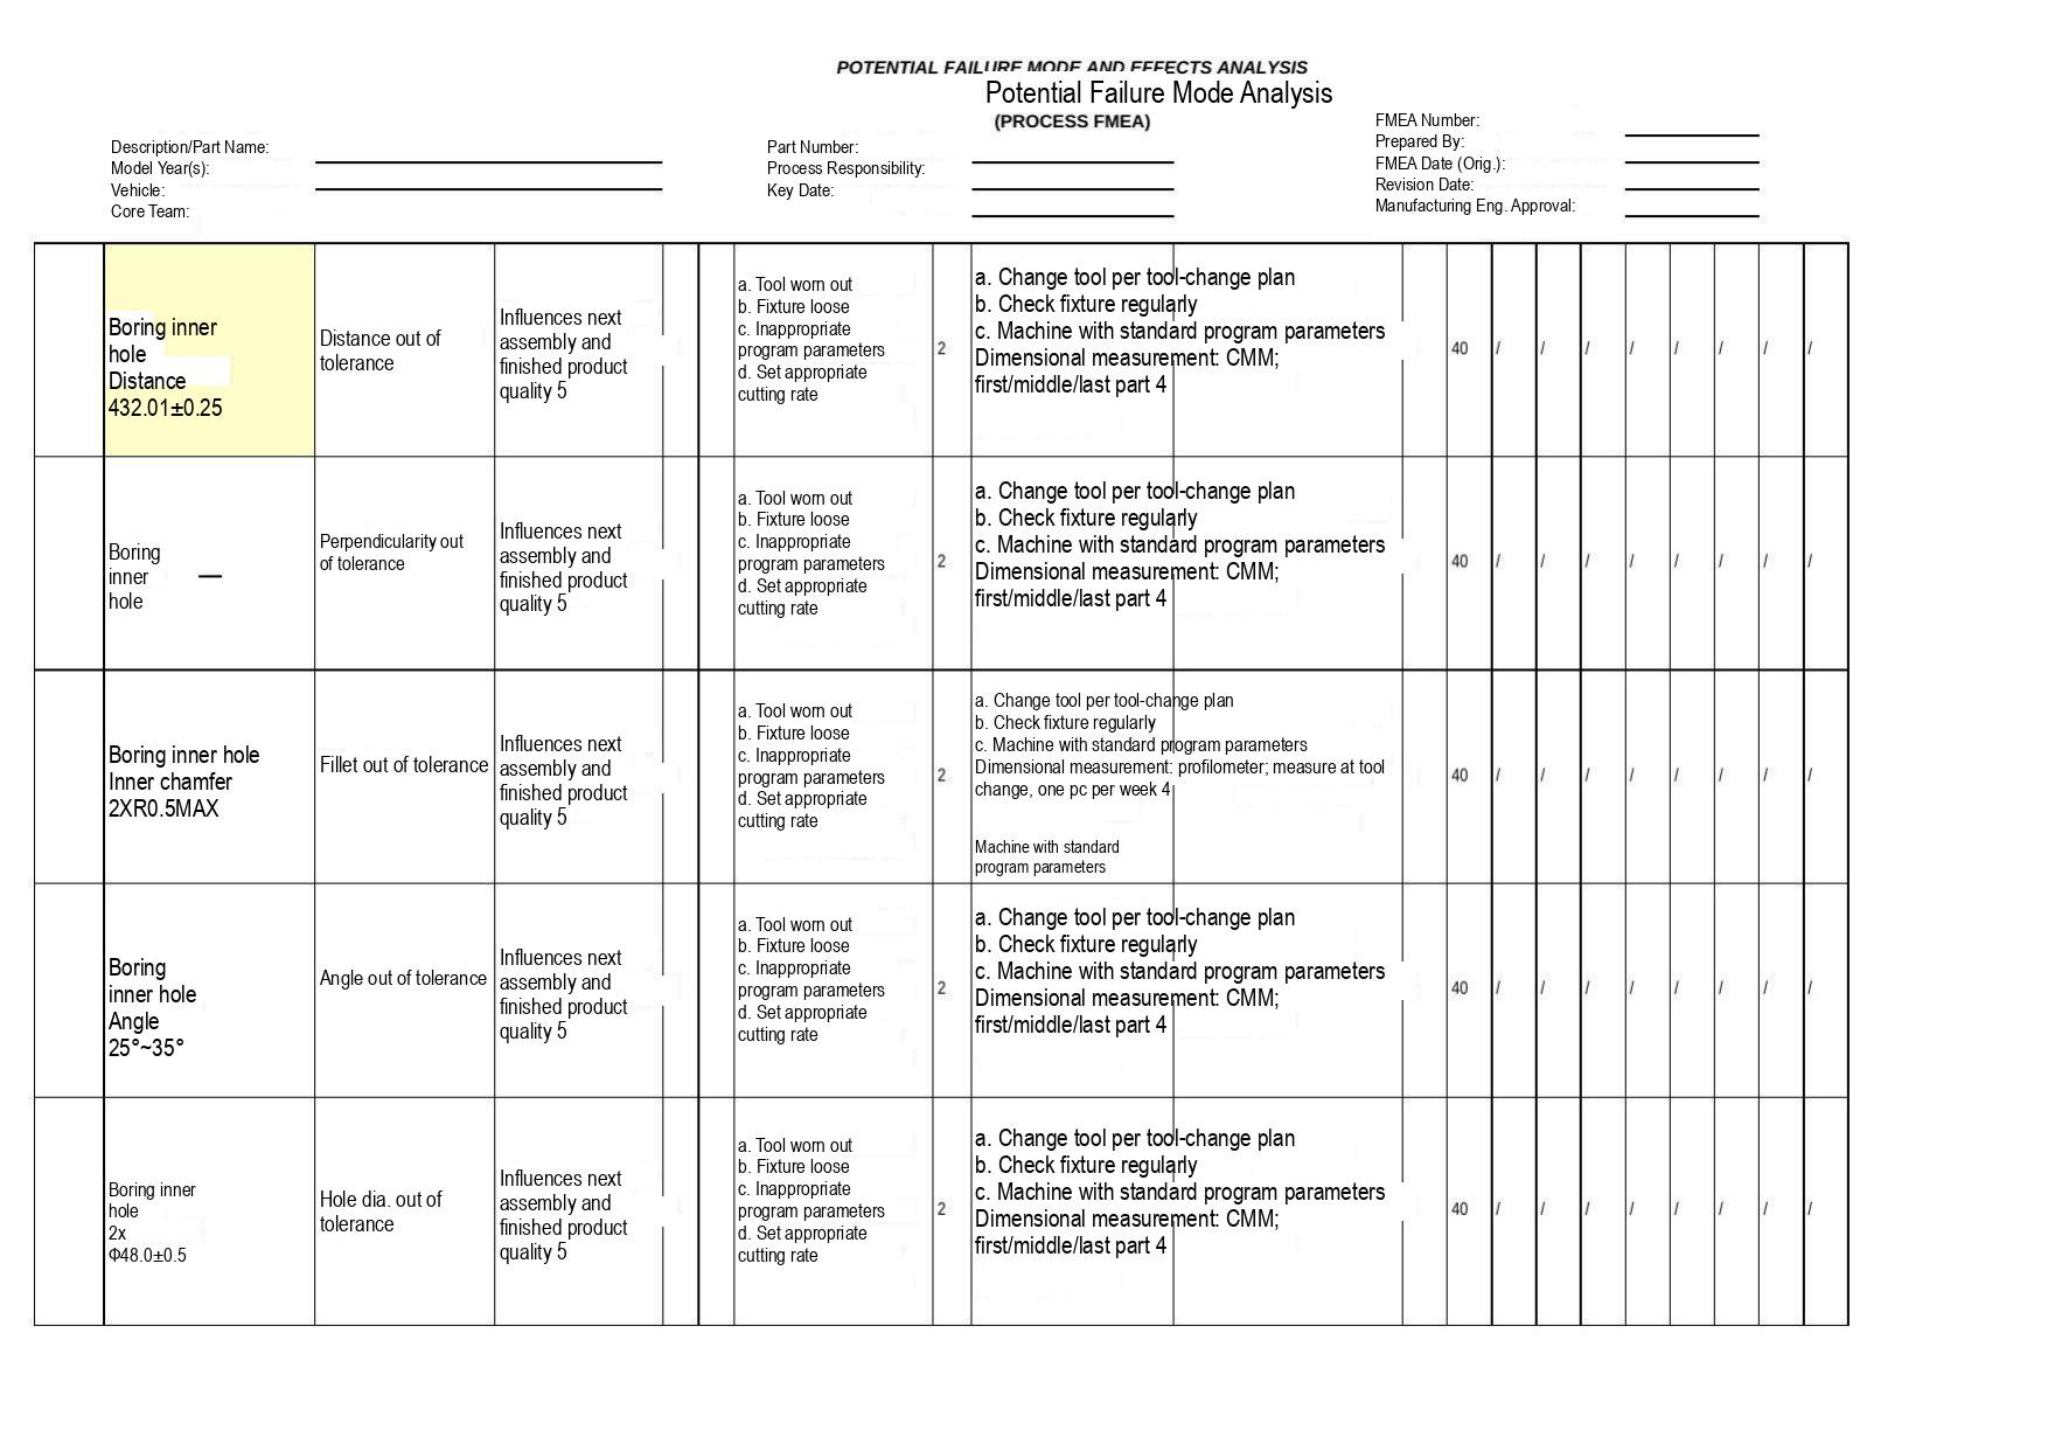**POTENTIAL FAILURE MODE AND EFFECTS ANALYSIS**

Potential Failure Mode Analysis

**(PROCESS FMEA)**

Description/Part Name:
Model Year(s):
Vehicle:
Core Team:

Part Number:
Process Responsibility:
Key Date:

FMEA Number:
Prepared By:
FMEA Date (Orig.):
Revision Date:
Manufacturing Eng. Approval:

| | | | | | | | | | | | | | | | | | | | |
|---|---|---|---|---|---|---|---|---|---|---|---|---|---|---|---|---|---|---|---|
| | Boring inner hole Distance 432.01±0.25 | Distance out of tolerance | Influences next assembly and finished product quality 5 | | | a. Tool worn out<br>b. Fixture loose<br>c. Inappropriate program parameters<br>d. Set appropriate cutting rate | 2 | a. Change tool per tool-change plan<br>b. Check fixture regularly<br>c. Machine with standard program parameters<br>Dimensional measurement: CMM; first/middle/last part 4 | | | 40 | / | / | / | / | / | / | / | / |
| | Boring inner hole — | Perpendicularity out of tolerance | Influences next assembly and finished product quality 5 | | | a. Tool worn out<br>b. Fixture loose<br>c. Inappropriate program parameters<br>d. Set appropriate cutting rate | 2 | a. Change tool per tool-change plan<br>b. Check fixture regularly<br>c. Machine with standard program parameters<br>Dimensional measurement: CMM; first/middle/last part 4 | | | 40 | / | / | / | / | / | / | / | / |
| | Boring inner hole Inner chamfer 2XR0.5MAX | Fillet out of tolerance | Influences next assembly and finished product quality 5 | | | a. Tool worn out<br>b. Fixture loose<br>c. Inappropriate program parameters<br>d. Set appropriate cutting rate | 2 | a. Change tool per tool-change plan<br>b. Check fixture regularly<br>c. Machine with standard program parameters<br>Dimensional measurement: profilometer; measure at tool change, one pc per week 4<br><br>Machine with standard program parameters | | | 40 | / | / | / | / | / | / | / | / |
| | Boring inner hole Angle 25°~35° | Angle out of tolerance | Influences next assembly and finished product quality 5 | | | a. Tool worn out<br>b. Fixture loose<br>c. Inappropriate program parameters<br>d. Set appropriate cutting rate | 2 | a. Change tool per tool-change plan<br>b. Check fixture regularly<br>c. Machine with standard program parameters<br>Dimensional measurement: CMM; first/middle/last part 4 | | | 40 | / | / | / | / | / | / | / | / |
| | Boring inner hole 2x Φ48.0±0.5 | Hole dia. out of tolerance | Influences next assembly and finished product quality 5 | | | a. Tool worn out<br>b. Fixture loose<br>c. Inappropriate program parameters<br>d. Set appropriate cutting rate | 2 | a. Change tool per tool-change plan<br>b. Check fixture regularly<br>c. Machine with standard program parameters<br>Dimensional measurement: CMM; first/middle/last part 4 | | | 40 | / | / | / | / | / | / | / | / |
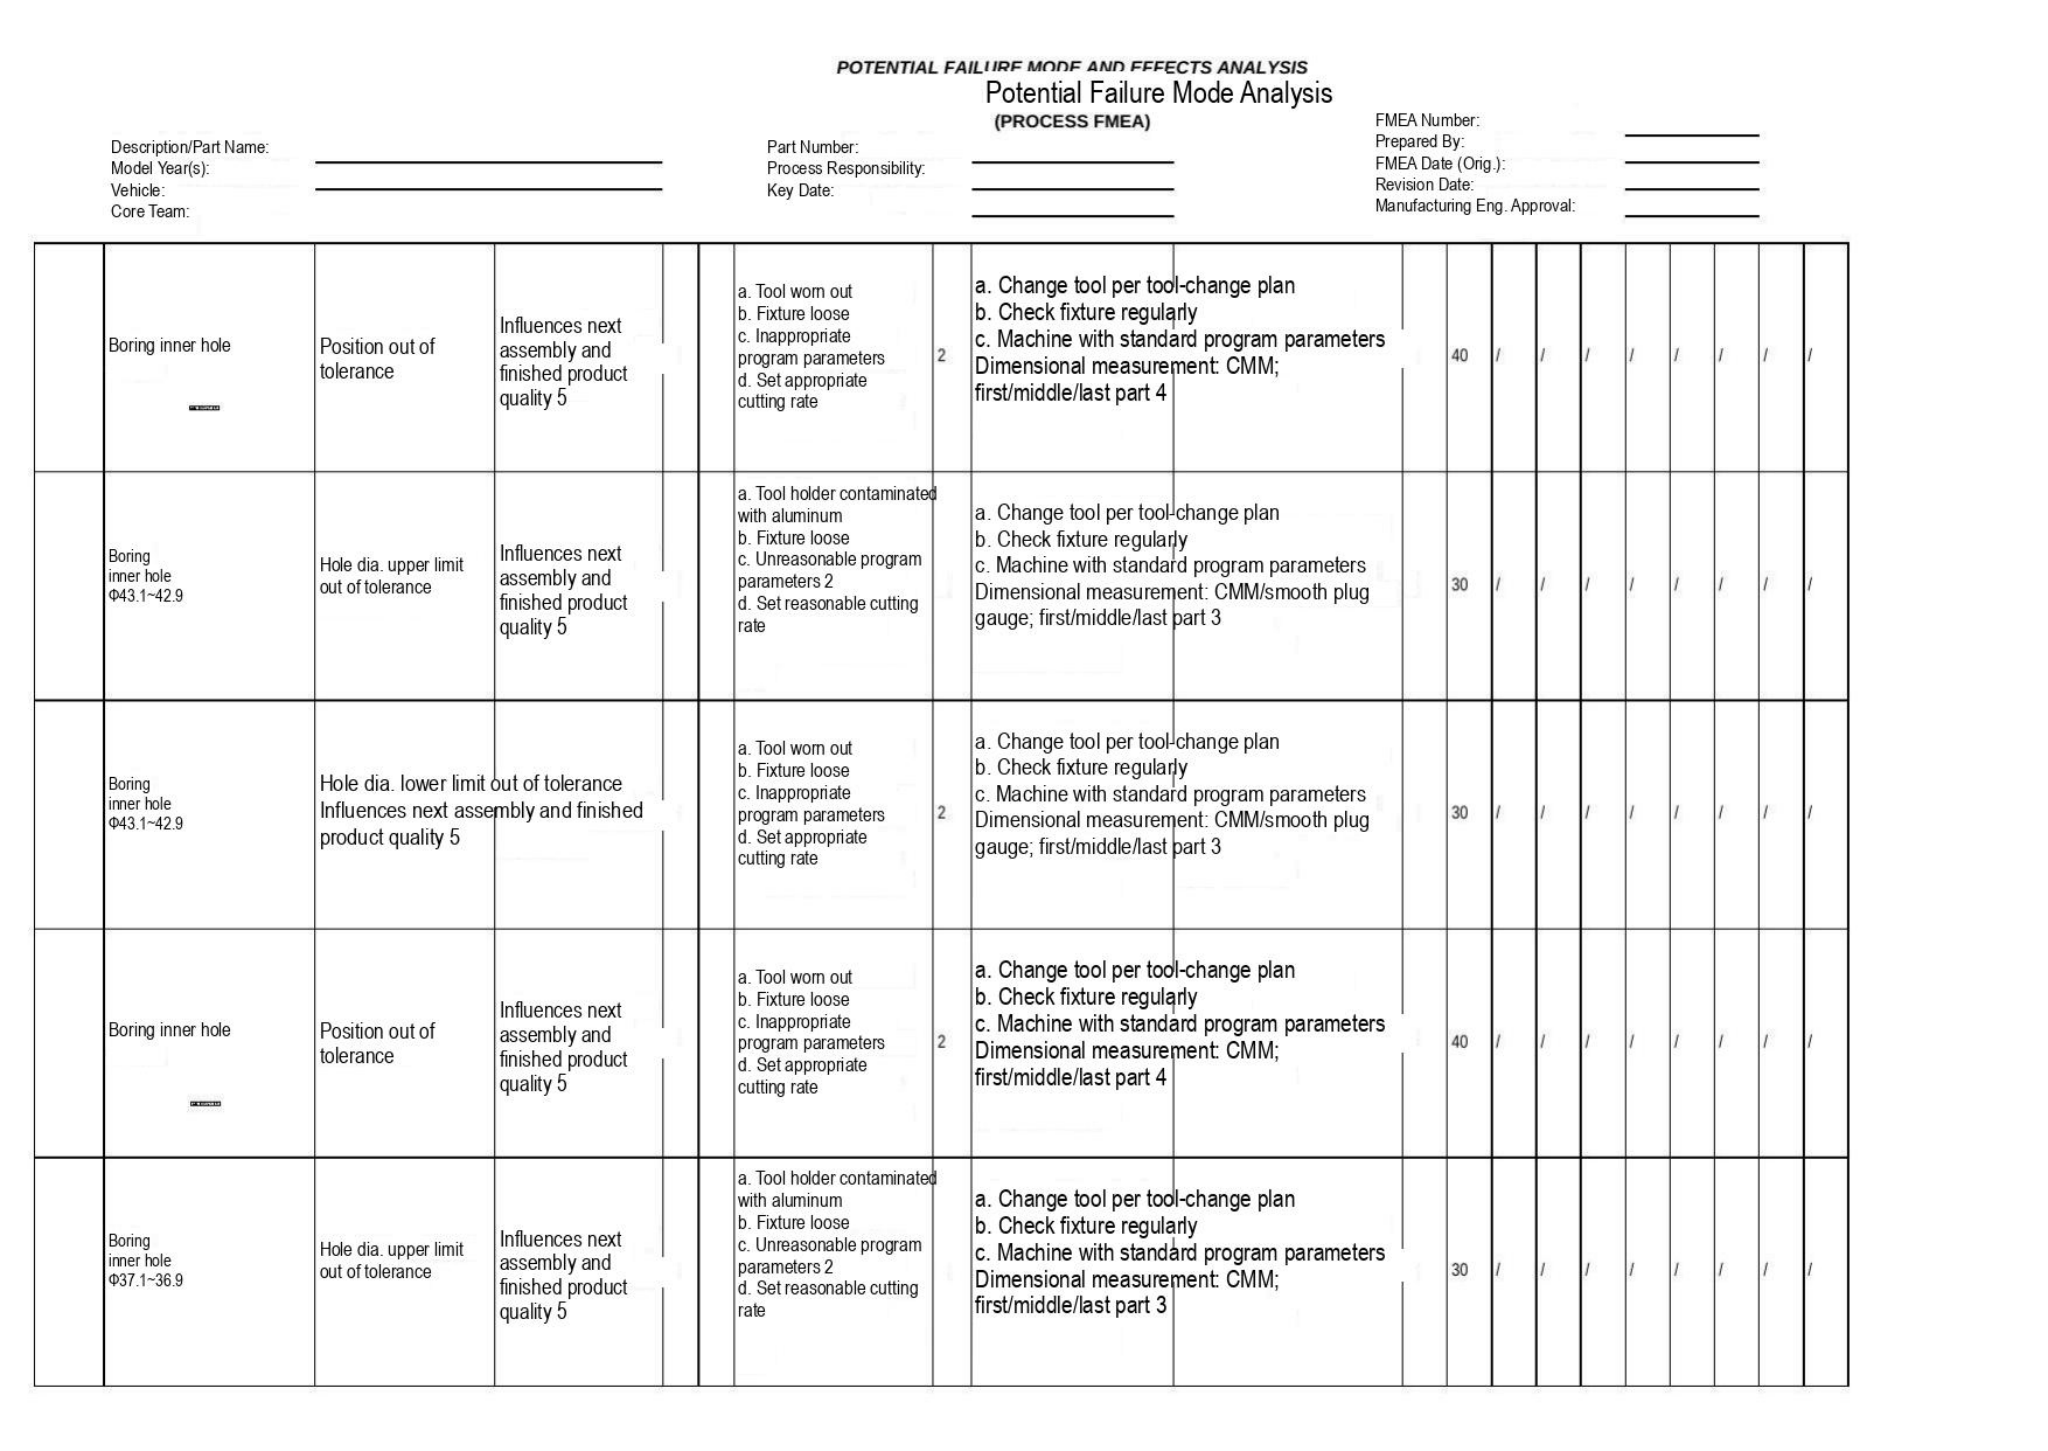**POTENTIAL FAILURE MODE AND EFFECTS ANALYSIS**
Potential Failure Mode Analysis
**(PROCESS FMEA)**

Description/Part Name:
Model Year(s):
Vehicle:
Core Team:

Part Number:
Process Responsibility:
Key Date:

FMEA Number:
Prepared By:
FMEA Date (Orig.):
Revision Date:
Manufacturing Eng. Approval:

| | | | | | | | | | | | | | | | | | | |
|---|---|---|---|---|---|---|---|---|---|---|---|---|---|---|---|---|---|---|
| | Boring inner hole | Position out of tolerance | Influences next assembly and finished product quality 5 | | | a. Tool worn out<br>b. Fixture loose<br>c. Inappropriate program parameters<br>d. Set appropriate cutting rate | 2 | a. Change tool per tool-change plan<br>b. Check fixture regularly<br>c. Machine with standard program parameters<br>Dimensional measurement: CMM; first/middle/last part 4 | | 40 | / | / | / | / | / | / | / | / |
| | Boring inner hole Φ43.1~42.9 | Hole dia. upper limit out of tolerance | Influences next assembly and finished product quality 5 | | | a. Tool holder contaminated with aluminum<br>b. Fixture loose<br>c. Unreasonable program parameters 2<br>d. Set reasonable cutting rate | | a. Change tool per tool-change plan<br>b. Check fixture regularly<br>c. Machine with standard program parameters<br>Dimensional measurement: CMM/smooth plug gauge; first/middle/last part 3 | | 30 | / | / | / | / | / | / | / | / |
| | Boring inner hole Φ43.1~42.9 | Hole dia. lower limit out of tolerance Influences next assembly and finished product quality 5 | | | | a. Tool worn out<br>b. Fixture loose<br>c. Inappropriate program parameters<br>d. Set appropriate cutting rate | 2 | a. Change tool per tool-change plan<br>b. Check fixture regularly<br>c. Machine with standard program parameters<br>Dimensional measurement: CMM/smooth plug gauge; first/middle/last part 3 | | 30 | / | / | / | / | / | / | / | / |
| | Boring inner hole | Position out of tolerance | Influences next assembly and finished product quality 5 | | | a. Tool worn out<br>b. Fixture loose<br>c. Inappropriate program parameters<br>d. Set appropriate cutting rate | 2 | a. Change tool per tool-change plan<br>b. Check fixture regularly<br>c. Machine with standard program parameters<br>Dimensional measurement: CMM; first/middle/last part 4 | | 40 | / | / | / | / | / | / | / | / |
| | Boring inner hole Φ37.1~36.9 | Hole dia. upper limit out of tolerance | Influences next assembly and finished product quality 5 | | | a. Tool holder contaminated with aluminum<br>b. Fixture loose<br>c. Unreasonable program parameters 2<br>d. Set reasonable cutting rate | | a. Change tool per tool-change plan<br>b. Check fixture regularly<br>c. Machine with standard program parameters<br>Dimensional measurement: CMM; first/middle/last part 3 | | 30 | / | / | / | / | / | / | / | / |
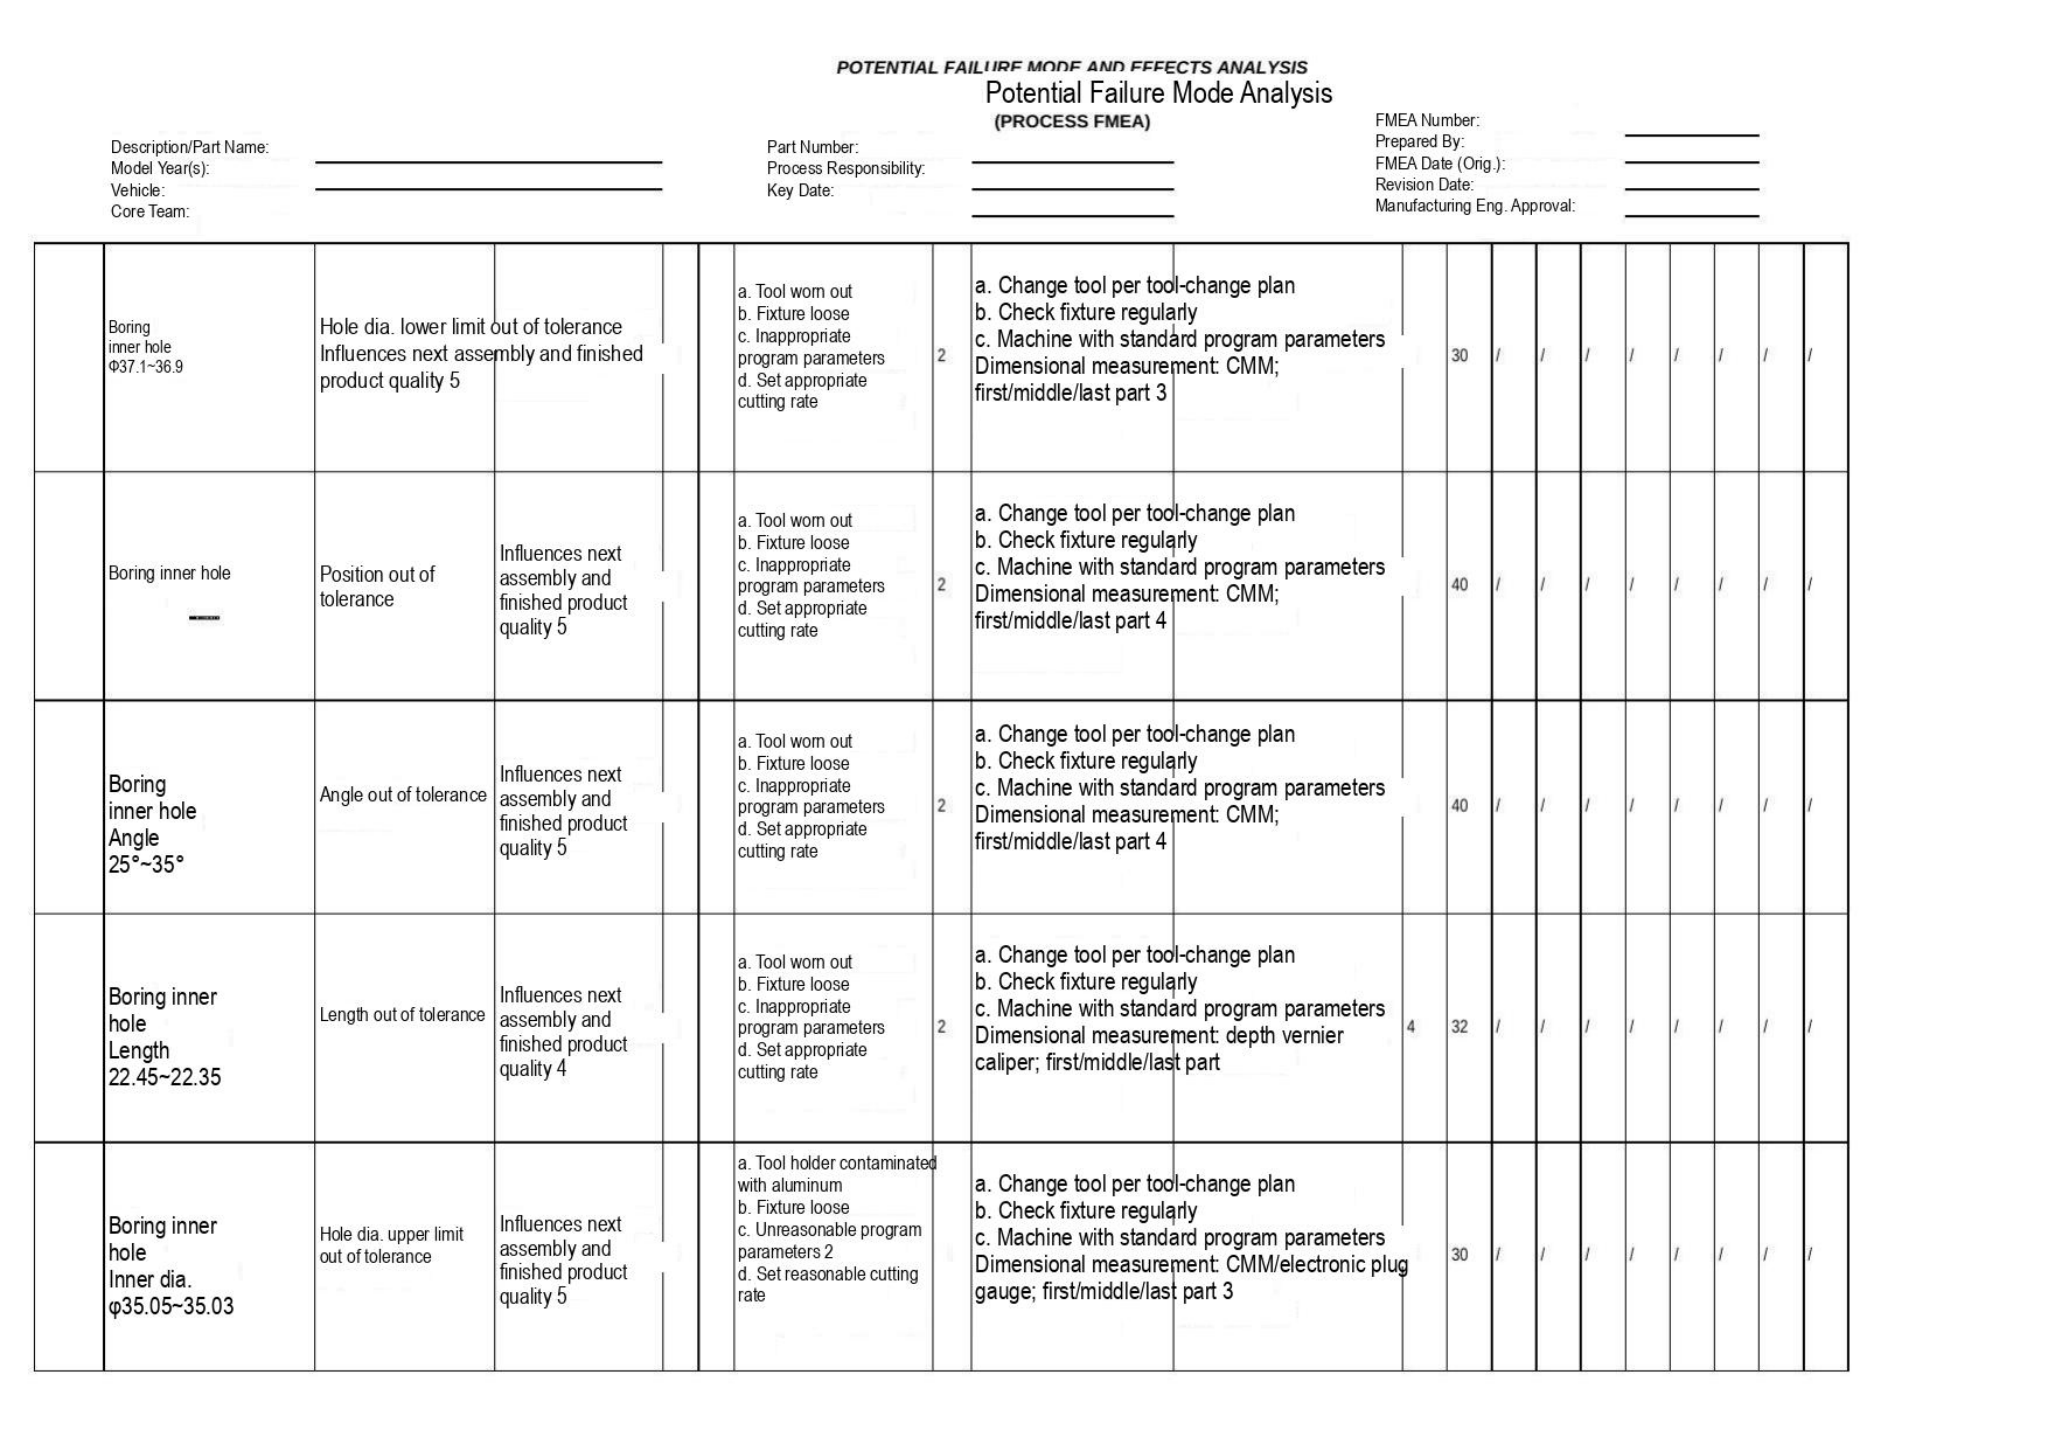**POTENTIAL FAILURE MODE AND EFFECTS ANALYSIS**

Potential Failure Mode Analysis

**(PROCESS FMEA)**

Description/Part Name:
Model Year(s):
Vehicle:
Core Team:

Part Number:
Process Responsibility:
Key Date:

FMEA Number:
Prepared By:
FMEA Date (Orig.):
Revision Date:
Manufacturing Eng. Approval:

| | | | | | | | | | | | | | | | | | | |
|---|---|---|---|---|---|---|---|---|---|---|---|---|---|---|---|---|---|---|
| | Boring inner hole Φ37.1~36.9 | Hole dia. lower limit out of tolerance Influences next assembly and finished product quality 5 | | | | a. Tool worn out b. Fixture loose c. Inappropriate program parameters d. Set appropriate cutting rate | 2 | a. Change tool per tool-change plan b. Check fixture regularly c. Machine with standard program parameters Dimensional measurement: CMM; first/middle/last part 3 | | 30 | / | / | / | / | / | / | / | / |
| | Boring inner hole | Position out of tolerance | Influences next assembly and finished product quality 5 | | | a. Tool worn out b. Fixture loose c. Inappropriate program parameters d. Set appropriate cutting rate | 2 | a. Change tool per tool-change plan b. Check fixture regularly c. Machine with standard program parameters Dimensional measurement: CMM; first/middle/last part 4 | | 40 | / | / | / | / | / | / | / | / |
| | Boring inner hole Angle 25°~35° | Angle out of tolerance | Influences next assembly and finished product quality 5 | | | a. Tool worn out b. Fixture loose c. Inappropriate program parameters d. Set appropriate cutting rate | 2 | a. Change tool per tool-change plan b. Check fixture regularly c. Machine with standard program parameters Dimensional measurement: CMM; first/middle/last part 4 | | 40 | / | / | / | / | / | / | / | / |
| | Boring inner hole Length 22.45~22.35 | Length out of tolerance | Influences next assembly and finished product quality 4 | | | a. Tool worn out b. Fixture loose c. Inappropriate program parameters d. Set appropriate cutting rate | 2 | a. Change tool per tool-change plan b. Check fixture regularly c. Machine with standard program parameters Dimensional measurement: depth vernier caliper; first/middle/last part | 4 | 32 | / | / | / | / | / | / | / | / |
| | Boring inner hole Inner dia. φ35.05~35.03 | Hole dia. upper limit out of tolerance | Influences next assembly and finished product quality 5 | | | a. Tool holder contaminated with aluminum b. Fixture loose c. Unreasonable program parameters 2 d. Set reasonable cutting rate | | a. Change tool per tool-change plan b. Check fixture regularly c. Machine with standard program parameters Dimensional measurement: CMM/electronic plug gauge; first/middle/last part 3 | | 30 | / | / | / | / | / | / | / | / |
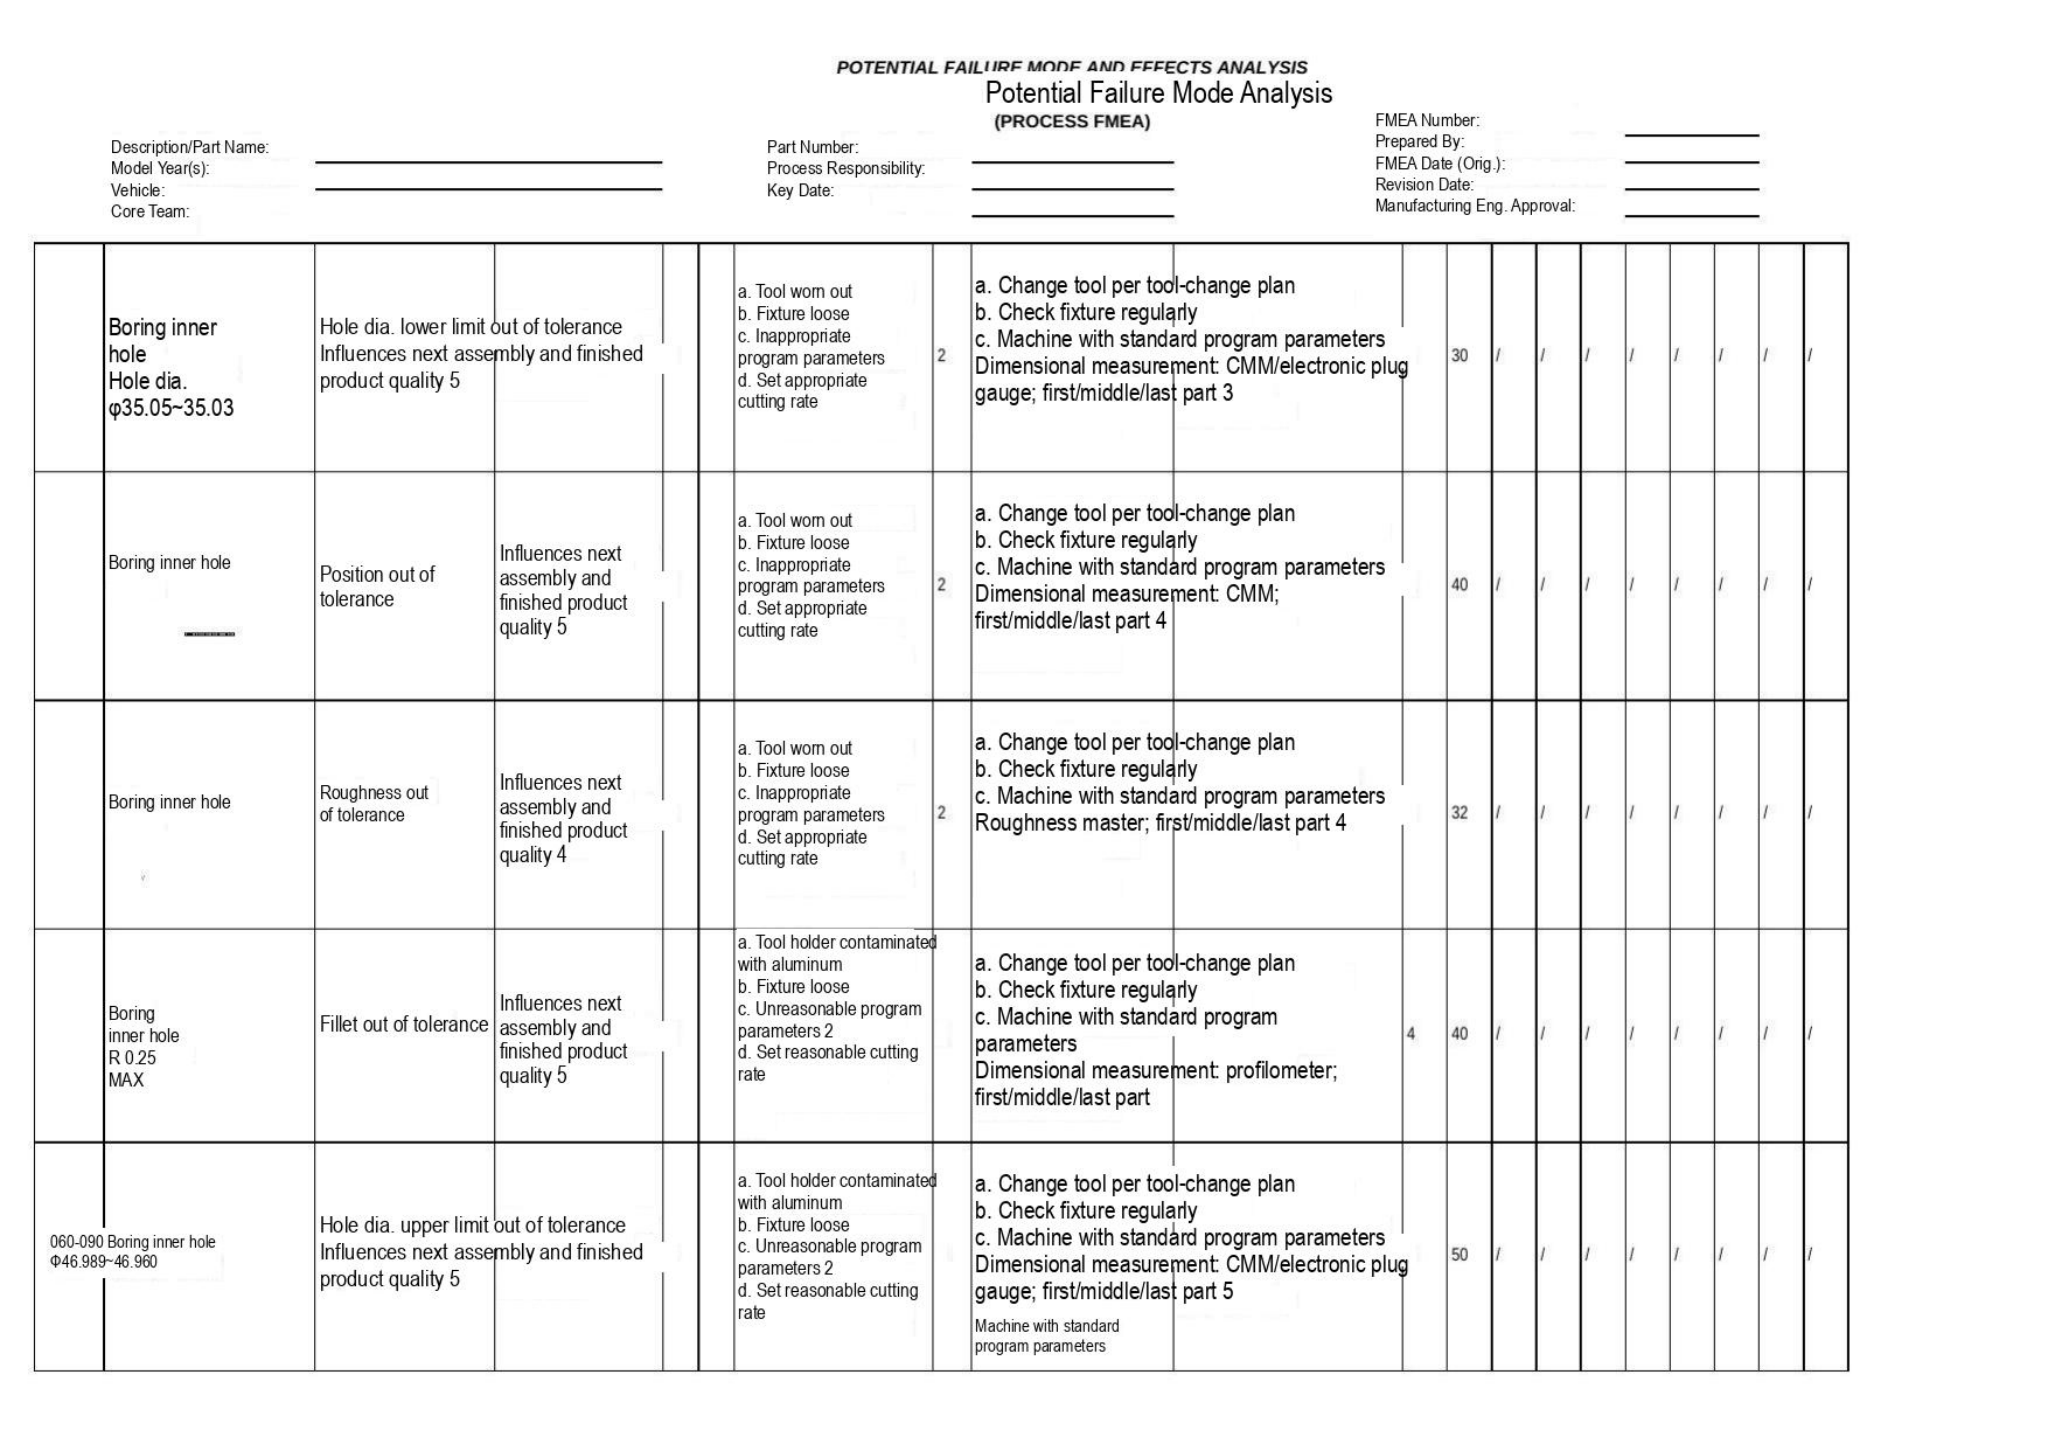**POTENTIAL FAILURE MODE AND EFFECTS ANALYSIS**

Potential Failure Mode Analysis

**(PROCESS FMEA)**

Description/Part Name:
Model Year(s):
Vehicle:
Core Team:

Part Number:
Process Responsibility:
Key Date:

FMEA Number:
Prepared By:
FMEA Date (Orig.):
Revision Date:
Manufacturing Eng. Approval:

| | | | | | | | | | | | | | | | | | | |
|---|---|---|---|---|---|---|---|---|---|---|---|---|---|---|---|---|---|---|
| | Boring inner hole Hole dia. φ35.05~35.03 | Hole dia. lower limit out of tolerance Influences next assembly and finished product quality 5 | | | | a. Tool worn out b. Fixture loose c. Inappropriate program parameters d. Set appropriate cutting rate | 2 | a. Change tool per tool-change plan b. Check fixture regularly c. Machine with standard program parameters Dimensional measurement: CMM/electronic plug gauge; first/middle/last part 3 | | 30 | / | / | / | / | / | / | / | / |
| | Boring inner hole | Position out of tolerance | Influences next assembly and finished product quality 5 | | | a. Tool worn out b. Fixture loose c. Inappropriate program parameters d. Set appropriate cutting rate | 2 | a. Change tool per tool-change plan b. Check fixture regularly c. Machine with standard program parameters Dimensional measurement: CMM; first/middle/last part 4 | | 40 | / | / | / | / | / | / | / | / |
| | Boring inner hole | Roughness out of tolerance | Influences next assembly and finished product quality 4 | | | a. Tool worn out b. Fixture loose c. Inappropriate program parameters d. Set appropriate cutting rate | 2 | a. Change tool per tool-change plan b. Check fixture regularly c. Machine with standard program parameters Roughness master; first/middle/last part 4 | | 32 | / | / | / | / | / | / | / | / |
| | Boring inner hole R 0.25 MAX | Fillet out of tolerance | Influences next assembly and finished product quality 5 | | | a. Tool holder contaminated with aluminum b. Fixture loose c. Unreasonable program parameters 2 d. Set reasonable cutting rate | | a. Change tool per tool-change plan b. Check fixture regularly c. Machine with standard program parameters Dimensional measurement: profilometer; first/middle/last part | 4 | 40 | / | / | / | / | / | / | / | / |
| 060-090 | Boring inner hole Φ46.989~46.960 | Hole dia. upper limit out of tolerance Influences next assembly and finished product quality 5 | | | | a. Tool holder contaminated with aluminum b. Fixture loose c. Unreasonable program parameters 2 d. Set reasonable cutting rate | | a. Change tool per tool-change plan b. Check fixture regularly c. Machine with standard program parameters Dimensional measurement: CMM/electronic plug gauge; first/middle/last part 5 Machine with standard program parameters | | 50 | / | / | / | / | / | / | / | / |
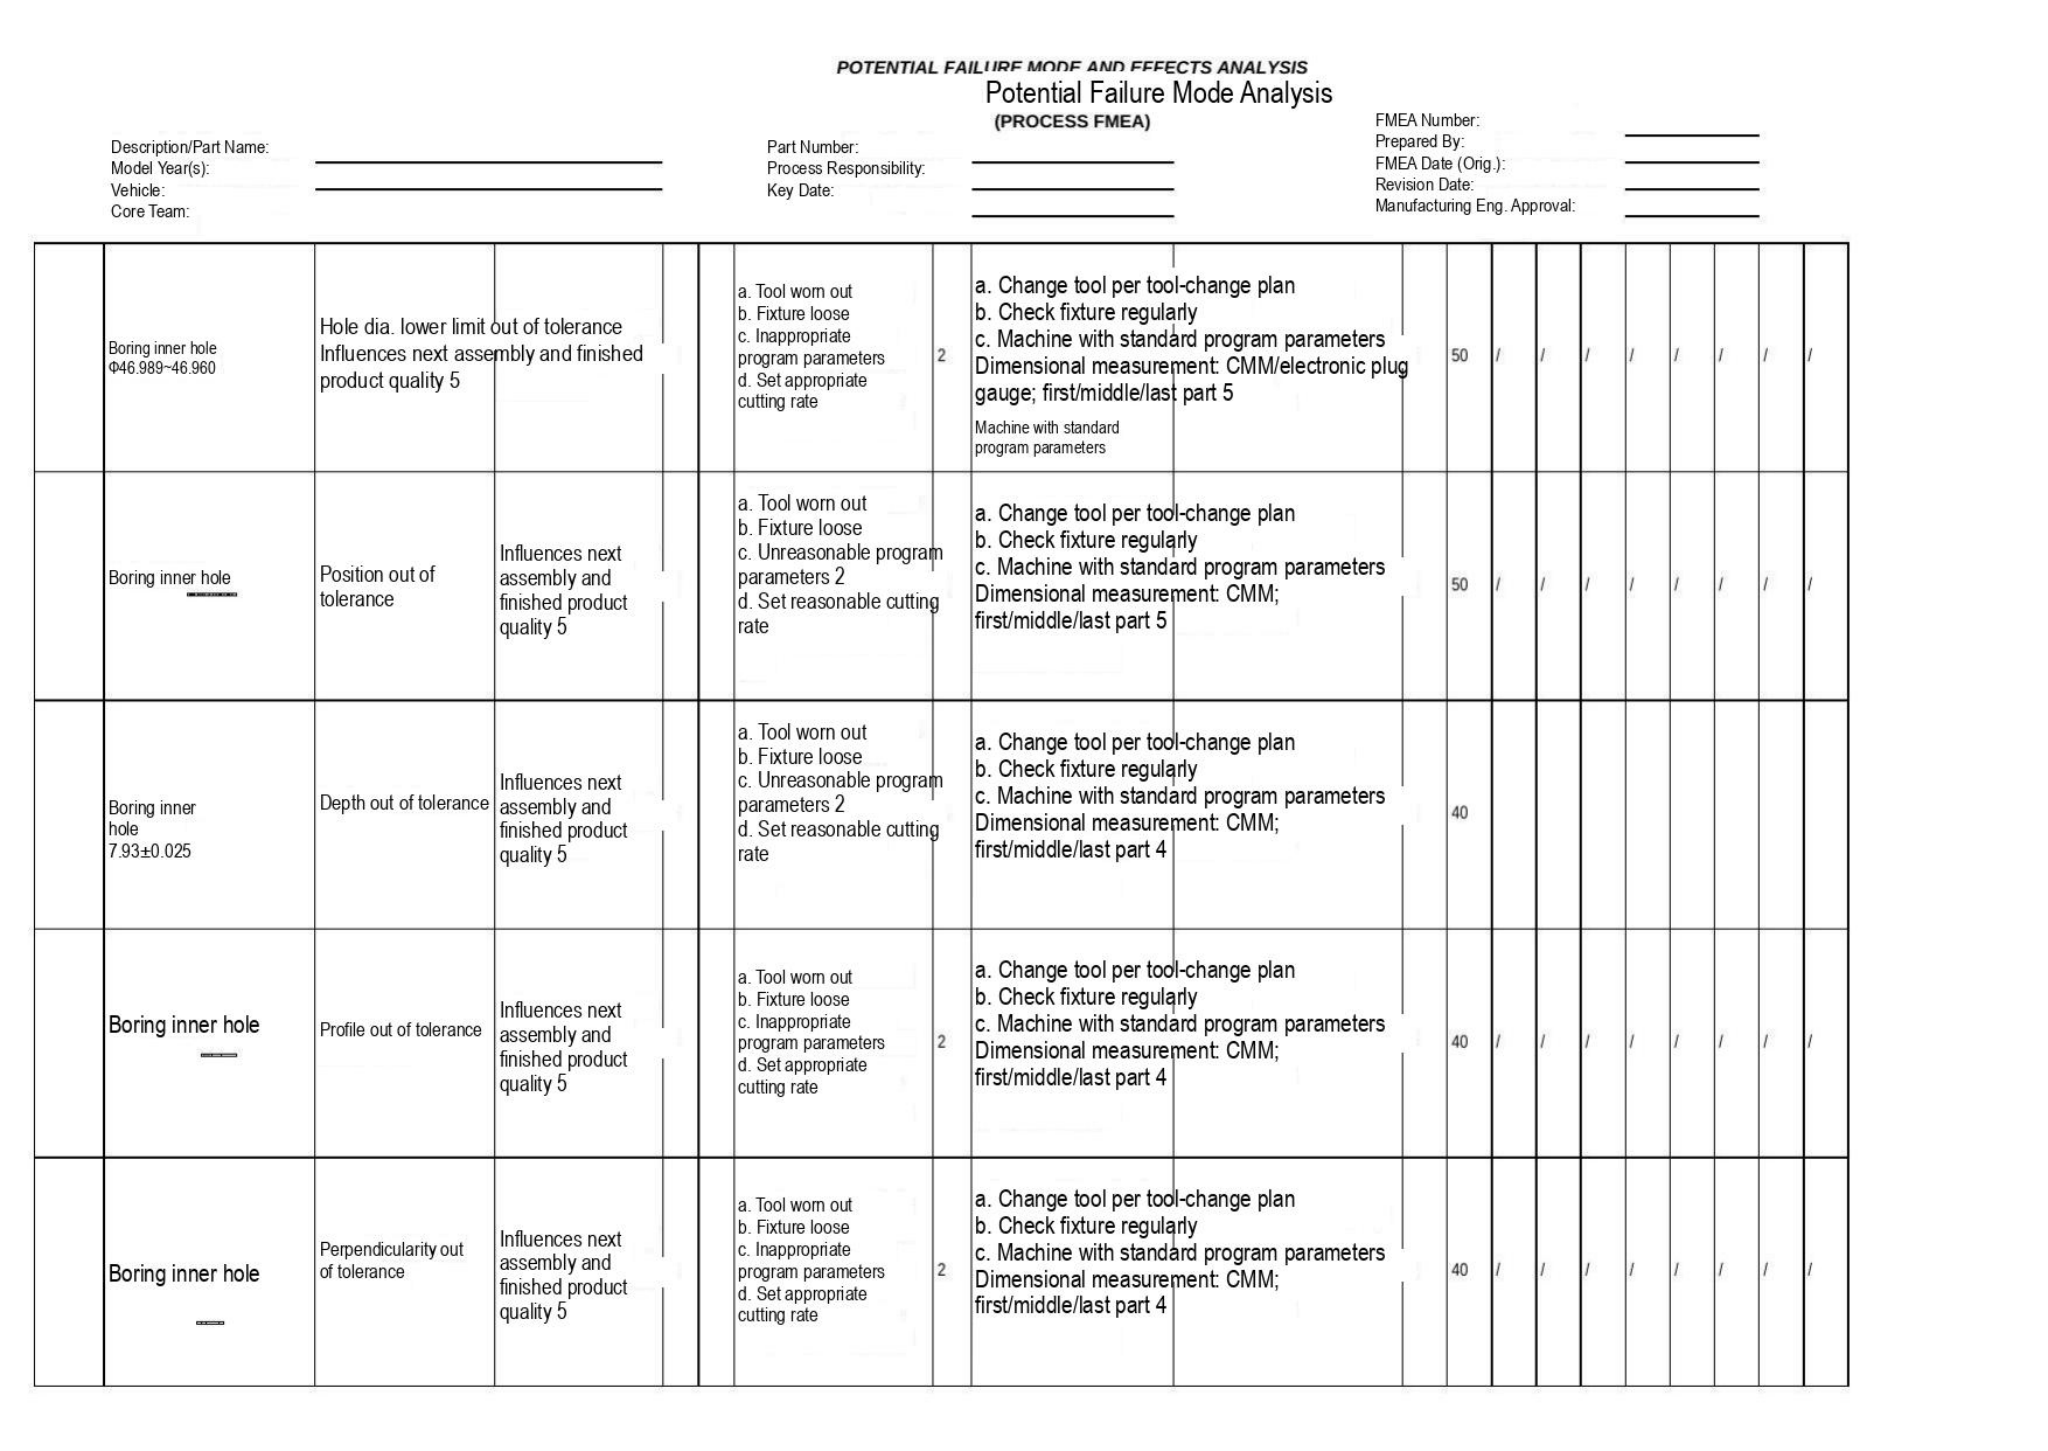**POTENTIAL FAILURE MODE AND EFFECTS ANALYSIS**
Potential Failure Mode Analysis
**(PROCESS FMEA)**

Description/Part Name:
Model Year(s):
Vehicle:
Core Team:

Part Number:
Process Responsibility:
Key Date:

FMEA Number:
Prepared By:
FMEA Date (Orig.):
Revision Date:
Manufacturing Eng. Approval:

| | | | | | | | | | | | | | | | | | | |
|---|---|---|---|---|---|---|---|---|---|---|---|---|---|---|---|---|---|---|
| | Boring inner hole Φ46.989~46.960 | Hole dia. lower limit out of tolerance Influences next assembly and finished product quality 5 | | | | a. Tool worn out b. Fixture loose c. Inappropriate program parameters d. Set appropriate cutting rate | 2 | a. Change tool per tool-change plan b. Check fixture regularly c. Machine with standard program parameters Dimensional measurement: CMM/electronic plug gauge; first/middle/last part 5 Machine with standard program parameters | | 50 | / | / | / | / | / | / | / | / |
| | Boring inner hole | Position out of tolerance | Influences next assembly and finished product quality 5 | | | a. Tool worn out b. Fixture loose c. Unreasonable program parameters 2 d. Set reasonable cutting rate | | a. Change tool per tool-change plan b. Check fixture regularly c. Machine with standard program parameters Dimensional measurement: CMM; first/middle/last part 5 | | 50 | / | / | / | / | / | / | / | / |
| | Boring inner hole 7.93±0.025 | Depth out of tolerance | Influences next assembly and finished product quality 5 | | | a. Tool worn out b. Fixture loose c. Unreasonable program parameters 2 d. Set reasonable cutting rate | | a. Change tool per tool-change plan b. Check fixture regularly c. Machine with standard program parameters Dimensional measurement: CMM; first/middle/last part 4 | | 40 | | | | | | | | |
| | Boring inner hole | Profile out of tolerance | Influences next assembly and finished product quality 5 | | | a. Tool worn out b. Fixture loose c. Inappropriate program parameters d. Set appropriate cutting rate | 2 | a. Change tool per tool-change plan b. Check fixture regularly c. Machine with standard program parameters Dimensional measurement: CMM; first/middle/last part 4 | | 40 | / | / | / | / | / | / | / | / |
| | Boring inner hole | Perpendicularity out of tolerance | Influences next assembly and finished product quality 5 | | | a. Tool worn out b. Fixture loose c. Inappropriate program parameters d. Set appropriate cutting rate | 2 | a. Change tool per tool-change plan b. Check fixture regularly c. Machine with standard program parameters Dimensional measurement: CMM; first/middle/last part 4 | | 40 | / | / | / | / | / | / | / | / |
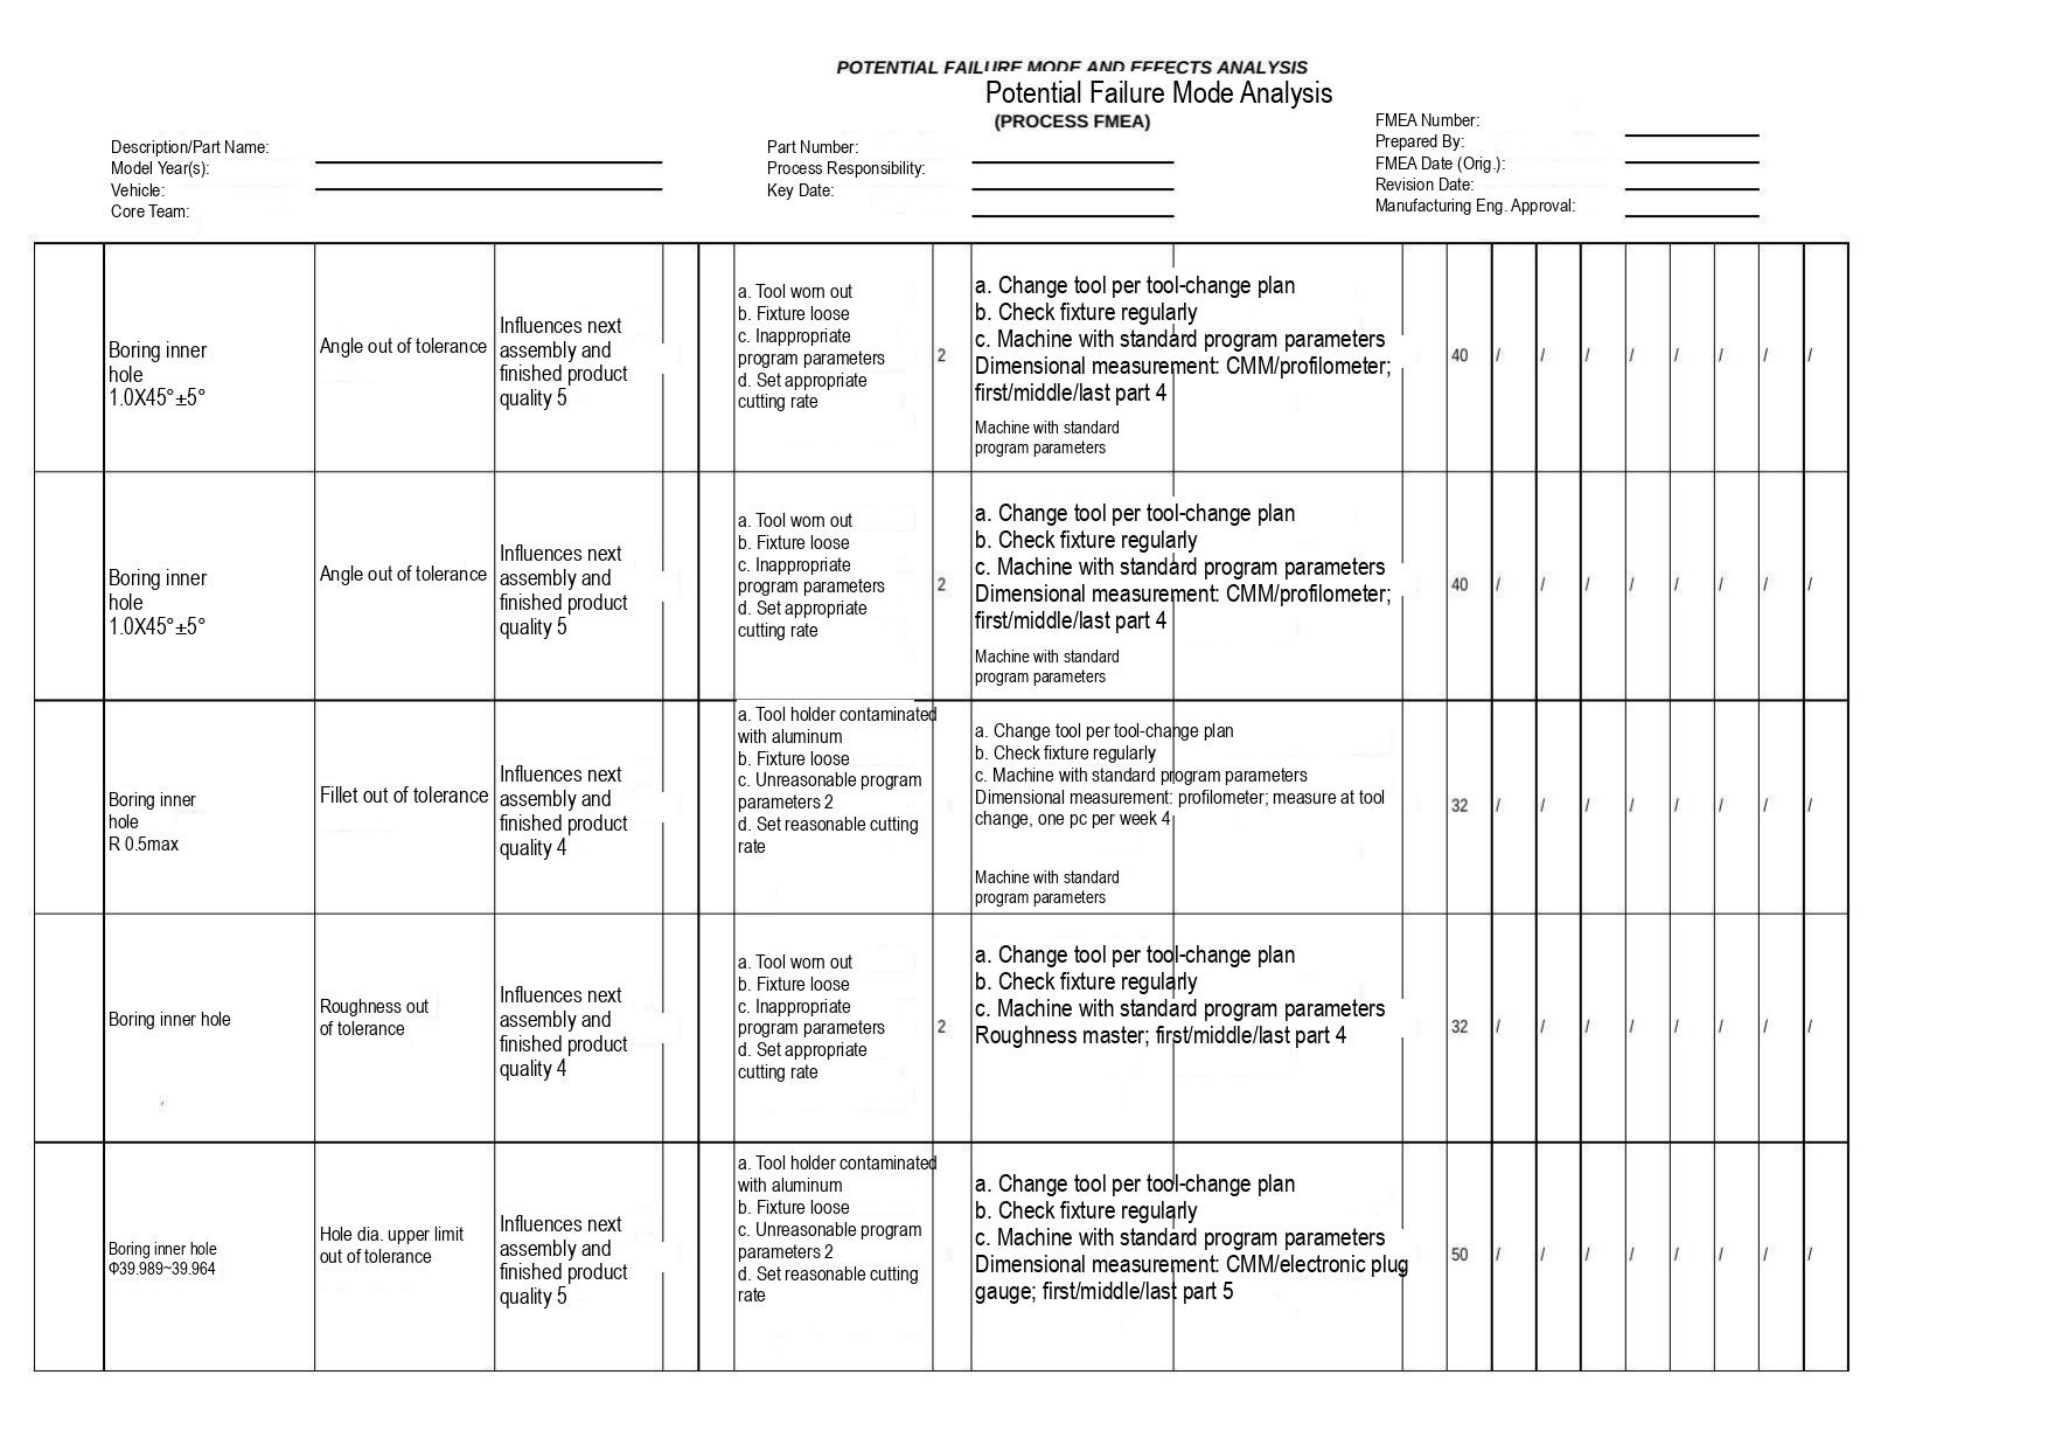POTENTIAL FAILURE MODE AND EFFECTS ANALYSIS

Potential Failure Mode Analysis

(PROCESS FMEA)

Description/Part Name:
Model Year(s):
Vehicle:
Core Team:

Part Number:
Process Responsibility:
Key Date:

FMEA Number:
Prepared By:
FMEA Date (Orig.):
Revision Date:
Manufacturing Eng. Approval:

| | | | | | | | | | | | | | | | | | | | |
|---|---|---|---|---|---|---|---|---|---|---|---|---|---|---|---|---|---|---|---|
| | Boring inner hole 1.0X45°±5° | Angle out of tolerance | Influences next assembly and finished product quality 5 | | | a. Tool worn out<br>b. Fixture loose<br>c. Inappropriate program parameters<br>d. Set appropriate cutting rate | 2 | a. Change tool per tool-change plan<br>b. Check fixture regularly<br>c. Machine with standard program parameters<br>Dimensional measurement: CMM/profilometer; first/middle/last part 4<br>Machine with standard program parameters | | 40 | / | / | / | / | / | / | / | / | |
| | Boring inner hole 1.0X45°±5° | Angle out of tolerance | Influences next assembly and finished product quality 5 | | | a. Tool worn out<br>b. Fixture loose<br>c. Inappropriate program parameters<br>d. Set appropriate cutting rate | 2 | a. Change tool per tool-change plan<br>b. Check fixture regularly<br>c. Machine with standard program parameters<br>Dimensional measurement: CMM/profilometer; first/middle/last part 4<br>Machine with standard program parameters | | 40 | / | / | / | / | / | / | / | / | |
| | Boring inner hole R 0.5max | Fillet out of tolerance | Influences next assembly and finished product quality 4 | | | a. Tool holder contaminated with aluminum<br>b. Fixture loose<br>c. Unreasonable program parameters 2<br>d. Set reasonable cutting rate | | a. Change tool per tool-change plan<br>b. Check fixture regularly<br>c. Machine with standard program parameters<br>Dimensional measurement: profilometer; measure at tool change, one pc per week 4<br>Machine with standard program parameters | | 32 | / | / | / | / | / | / | / | / | |
| | Boring inner hole | Roughness out of tolerance | Influences next assembly and finished product quality 4 | | | a. Tool worn out<br>b. Fixture loose<br>c. Inappropriate program parameters<br>d. Set appropriate cutting rate | 2 | a. Change tool per tool-change plan<br>b. Check fixture regularly<br>c. Machine with standard program parameters<br>Roughness master; first/middle/last part 4 | | 32 | / | / | / | / | / | / | / | / | |
| | Boring inner hole Φ39.989~39.964 | Hole dia. upper limit out of tolerance | Influences next assembly and finished product quality 5 | | | a. Tool holder contaminated with aluminum<br>b. Fixture loose<br>c. Unreasonable program parameters 2<br>d. Set reasonable cutting rate | | a. Change tool per tool-change plan<br>b. Check fixture regularly<br>c. Machine with standard program parameters<br>Dimensional measurement: CMM/electronic plug gauge; first/middle/last part 5 | | 50 | / | / | / | / | / | / | / | / | |